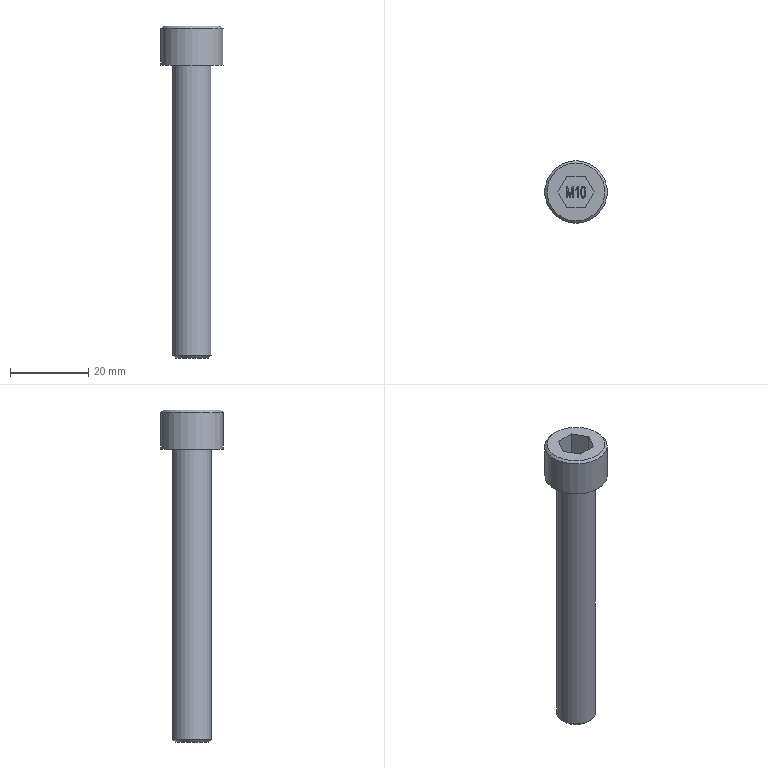Part | STEP file | EM11007500 | 1 solid | 42 faces | box 16 x 16 x 85 mm | volume 7551 mm3 | plane 30 | other 8 | cylinder 2 | cone 2 | commonest cylinder face diameters 10 x1 16 x1